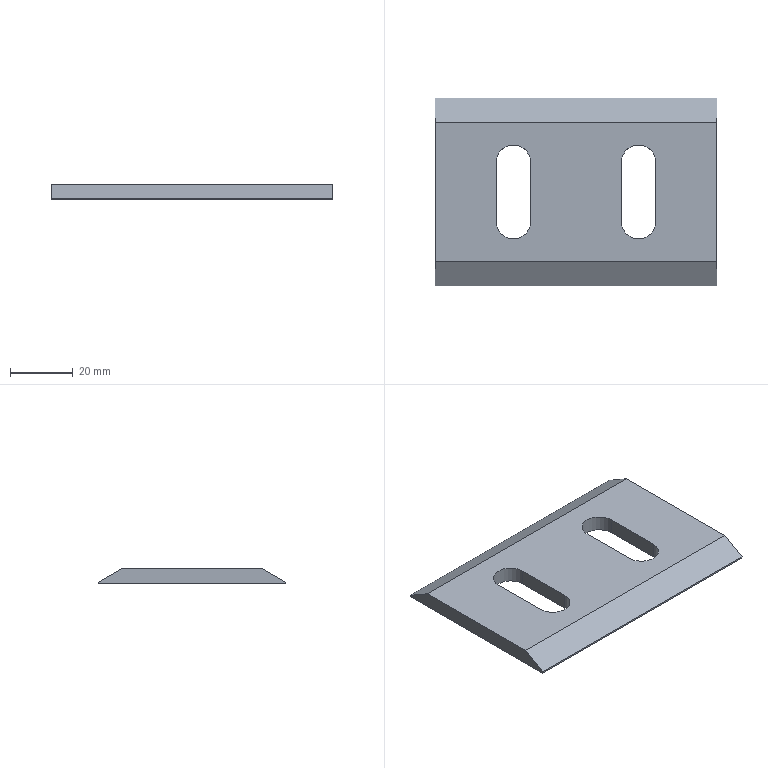Part | SolidWorks | features Chamfer 2, FlatPattern 1, SMBaseFlange 1, SheetMetal 1 | 1 solid | 16 faces | box 90 x 60 x 5 mm | volume 20803 mm3 | plane 12 | cylinder 4 | commonest cylinder face diameters 11 x4
STEP:
#1=CARTESIAN_POINT('',(0.,0.,-5.));
#2=VERTEX_POINT('',#1);
#3=CARTESIAN_POINT('',(0.,0.,-4.5));
#4=VERTEX_POINT('',#3);
#5=CARTESIAN_POINT('',(0.,0.,-5.));
#6=DIRECTION('',(0.,0.,1.));
#7=VECTOR('',#6,1000.);
#8=LINE('',#5,#7);
#9=EDGE_CURVE('',#2,#4,#8,.T.);
#10=ORIENTED_EDGE('',*,*,#9,.T.);
#11=CARTESIAN_POINT('',(0.,7.794,0.));
#12=VERTEX_POINT('',#11);
#13=CARTESIAN_POINT('',(0.,-0.2165,-4.625));
#14=DIRECTION('',(0.,0.866,0.5));
#15=VECTOR('',#14,1000.);
#16=LINE('',#13,#15);
#17=EDGE_CURVE('',#4,#12,#16,.T.);
#18=ORIENTED_EDGE('',*,*,#17,.T.);
#19=CARTESIAN_POINT('',(0.,52.206,0.));
#20=VERTEX_POINT('',#19);
#21=CARTESIAN_POINT('',(0.,0.,0.));
#22=DIRECTION('',(0.,-1.,0.));
#23=VECTOR('',#22,1000.);
#24=LINE('',#21,#23);
#25=EDGE_CURVE('',#20,#12,#24,.T.);
#26=ORIENTED_EDGE('',*,*,#25,.F.);
#27=CARTESIAN_POINT('',(0.,60.,-4.5));
#28=VERTEX_POINT('',#27);
#29=CARTESIAN_POINT('',(0.,15.217,21.356));
#30=DIRECTION('',(0.,0.866,-0.5));
#31=VECTOR('',#30,1000.);
#32=LINE('',#29,#31);
#33=EDGE_CURVE('',#20,#28,#32,.T.);
#34=ORIENTED_EDGE('',*,*,#33,.T.);
#35=CARTESIAN_POINT('',(0.,60.,-5.));
#36=VERTEX_POINT('',#35);
#37=CARTESIAN_POINT('',(0.,60.,-5.));
#38=DIRECTION('',(0.,0.,1.));
#39=VECTOR('',#38,1000.);
#40=LINE('',#37,#39);
#41=EDGE_CURVE('',#36,#28,#40,.T.);
#42=ORIENTED_EDGE('',*,*,#41,.F.);
#43=CARTESIAN_POINT('',(0.,0.,-5.));
#44=DIRECTION('',(0.,-1.,0.));
#45=VECTOR('',#44,1000.);
#46=LINE('',#43,#45);
#47=EDGE_CURVE('',#36,#2,#46,.T.);
#48=ORIENTED_EDGE('',*,*,#47,.T.);
#49=EDGE_LOOP('',(#10,#18,#26,#34,#42,#48));
#50=FACE_OUTER_BOUND('',#49,.T.);
#51=CARTESIAN_POINT('',(0.,0.,-5.));
#52=DIRECTION('',(-1.,0.,0.));
#53=DIRECTION('',(0.,0.,1.));
#54=AXIS2_PLACEMENT_3D('',#51,#52,#53);
#55=PLANE('',#54);
#56=ADVANCED_FACE('',(#50),#55,.T.);
#57=ORIENTED_EDGE('',*,*,#41,.T.);
#58=CARTESIAN_POINT('',(90.,60.,-4.5));
#59=VERTEX_POINT('',#58);
#60=CARTESIAN_POINT('',(90.,60.,-4.5));
#61=DIRECTION('',(1.,0.,0.));
#62=VECTOR('',#61,1000.);
#63=LINE('',#60,#62);
#64=EDGE_CURVE('',#28,#59,#63,.T.);
#65=ORIENTED_EDGE('',*,*,#64,.T.);
#66=CARTESIAN_POINT('',(90.,60.,-5.));
#67=VERTEX_POINT('',#66);
#68=CARTESIAN_POINT('',(90.,60.,-5.));
#69=DIRECTION('',(0.,0.,1.));
#70=VECTOR('',#69,1000.);
#71=LINE('',#68,#70);
#72=EDGE_CURVE('',#67,#59,#71,.T.);
#73=ORIENTED_EDGE('',*,*,#72,.F.);
#74=CARTESIAN_POINT('',(0.,60.,-5.));
#75=DIRECTION('',(-1.,0.,0.));
#76=VECTOR('',#75,1000.);
#77=LINE('',#74,#76);
#78=EDGE_CURVE('',#67,#36,#77,.T.);
#79=ORIENTED_EDGE('',*,*,#78,.T.);
#80=EDGE_LOOP('',(#57,#65,#73,#79));
#81=FACE_OUTER_BOUND('',#80,.T.);
#82=CARTESIAN_POINT('',(0.,60.,-5.));
#83=DIRECTION('',(0.,1.,0.));
#84=DIRECTION('',(0.,0.,1.));
#85=AXIS2_PLACEMENT_3D('',#82,#83,#84);
#86=PLANE('',#85);
#87=ADVANCED_FACE('',(#81),#86,.T.);
#88=CARTESIAN_POINT('',(90.,7.794,0.));
#89=VERTEX_POINT('',#88);
#90=CARTESIAN_POINT('',(90.,52.206,0.));
#91=VERTEX_POINT('',#90);
#92=CARTESIAN_POINT('',(90.,0.,0.));
#93=DIRECTION('',(0.,1.,0.));
#94=VECTOR('',#93,1000.);
#95=LINE('',#92,#94);
#96=EDGE_CURVE('',#89,#91,#95,.T.);
#97=ORIENTED_EDGE('',*,*,#96,.F.);
#98=CARTESIAN_POINT('',(90.,0.,-4.5));
#99=VERTEX_POINT('',#98);
#100=CARTESIAN_POINT('',(90.,-0.2165,-4.625));
#101=DIRECTION('',(0.,-0.866,-0.5));
#102=VECTOR('',#101,1000.);
#103=LINE('',#100,#102);
#104=EDGE_CURVE('',#89,#99,#103,.T.);
#105=ORIENTED_EDGE('',*,*,#104,.T.);
#106=CARTESIAN_POINT('',(90.,0.,-5.));
#107=VERTEX_POINT('',#106);
#108=CARTESIAN_POINT('',(90.,0.,-5.));
#109=DIRECTION('',(0.,0.,1.));
#110=VECTOR('',#109,1000.);
#111=LINE('',#108,#110);
#112=EDGE_CURVE('',#107,#99,#111,.T.);
#113=ORIENTED_EDGE('',*,*,#112,.F.);
#114=CARTESIAN_POINT('',(90.,0.,-5.));
#115=DIRECTION('',(0.,1.,0.));
#116=VECTOR('',#115,1000.);
#117=LINE('',#114,#116);
#118=EDGE_CURVE('',#107,#67,#117,.T.);
#119=ORIENTED_EDGE('',*,*,#118,.T.);
#120=ORIENTED_EDGE('',*,*,#72,.T.);
#121=CARTESIAN_POINT('',(90.,15.217,21.356));
#122=DIRECTION('',(0.,-0.866,0.5));
#123=VECTOR('',#122,1000.);
#124=LINE('',#121,#123);
#125=EDGE_CURVE('',#59,#91,#124,.T.);
#126=ORIENTED_EDGE('',*,*,#125,.T.);
#127=EDGE_LOOP('',(#97,#105,#113,#119,#120,#126));
#128=FACE_OUTER_BOUND('',#127,.T.);
#129=CARTESIAN_POINT('',(90.,0.,-5.));
#130=DIRECTION('',(1.,0.,0.));
#131=DIRECTION('',(0.,0.,-1.));
#132=AXIS2_PLACEMENT_3D('',#129,#130,#131);
#133=PLANE('',#132);
#134=ADVANCED_FACE('',(#128),#133,.T.);
#135=ORIENTED_EDGE('',*,*,#112,.T.);
#136=CARTESIAN_POINT('',(0.,0.,-4.5));
#137=DIRECTION('',(-1.,0.,0.));
#138=VECTOR('',#137,1000.);
#139=LINE('',#136,#138);
#140=EDGE_CURVE('',#99,#4,#139,.T.);
#141=ORIENTED_EDGE('',*,*,#140,.T.);
#142=ORIENTED_EDGE('',*,*,#9,.F.);
#143=CARTESIAN_POINT('',(0.,0.,-5.));
#144=DIRECTION('',(1.,0.,0.));
#145=VECTOR('',#144,1000.);
#146=LINE('',#143,#145);
#147=EDGE_CURVE('',#2,#107,#146,.T.);
#148=ORIENTED_EDGE('',*,*,#147,.T.);
#149=EDGE_LOOP('',(#135,#141,#142,#148));
#150=FACE_OUTER_BOUND('',#149,.T.);
#151=CARTESIAN_POINT('',(0.,0.,-5.));
#152=DIRECTION('',(0.,-1.,0.));
#153=DIRECTION('',(0.,0.,-1.));
#154=AXIS2_PLACEMENT_3D('',#151,#152,#153);
#155=PLANE('',#154);
#156=ADVANCED_FACE('',(#150),#155,.T.);
#157=CARTESIAN_POINT('',(70.5,39.5,-5.));
#158=VERTEX_POINT('',#157);
#159=CARTESIAN_POINT('',(59.5,39.5,-5.));
#160=VERTEX_POINT('',#159);
#161=CARTESIAN_POINT('',(65.,39.5,-5.));
#162=DIRECTION('',(0.,0.,1.));
#163=DIRECTION('',(1.,0.,0.));
#164=AXIS2_PLACEMENT_3D('',#161,#162,#163);
#165=CIRCLE('',#164,5.5);
#166=EDGE_CURVE('',#158,#160,#165,.T.);
#167=ORIENTED_EDGE('',*,*,#166,.T.);
#168=CARTESIAN_POINT('',(59.5,20.5,-5.));
#169=VERTEX_POINT('',#168);
#170=CARTESIAN_POINT('',(59.5,39.5,-5.));
#171=DIRECTION('',(0.,-1.,0.));
#172=VECTOR('',#171,1000.);
#173=LINE('',#170,#172);
#174=EDGE_CURVE('',#160,#169,#173,.T.);
#175=ORIENTED_EDGE('',*,*,#174,.T.);
#176=CARTESIAN_POINT('',(70.5,20.5,-5.));
#177=VERTEX_POINT('',#176);
#178=CARTESIAN_POINT('',(65.,20.5,-5.));
#179=DIRECTION('',(0.,0.,1.));
#180=DIRECTION('',(1.,0.,0.));
#181=AXIS2_PLACEMENT_3D('',#178,#179,#180);
#182=CIRCLE('',#181,5.5);
#183=EDGE_CURVE('',#169,#177,#182,.T.);
#184=ORIENTED_EDGE('',*,*,#183,.T.);
#185=CARTESIAN_POINT('',(70.5,39.5,-5.));
#186=DIRECTION('',(0.,1.,0.));
#187=VECTOR('',#186,1000.);
#188=LINE('',#185,#187);
#189=EDGE_CURVE('',#177,#158,#188,.T.);
#190=ORIENTED_EDGE('',*,*,#189,.T.);
#191=EDGE_LOOP('',(#167,#175,#184,#190));
#192=FACE_BOUND('',#191,.T.);
#193=CARTESIAN_POINT('',(30.5,39.5,-5.));
#194=VERTEX_POINT('',#193);
#195=CARTESIAN_POINT('',(19.5,39.5,-5.));
#196=VERTEX_POINT('',#195);
#197=CARTESIAN_POINT('',(25.,39.5,-5.));
#198=DIRECTION('',(0.,0.,1.));
#199=DIRECTION('',(1.,0.,0.));
#200=AXIS2_PLACEMENT_3D('',#197,#198,#199);
#201=CIRCLE('',#200,5.5);
#202=EDGE_CURVE('',#194,#196,#201,.T.);
#203=ORIENTED_EDGE('',*,*,#202,.T.);
#204=CARTESIAN_POINT('',(19.5,20.5,-5.));
#205=VERTEX_POINT('',#204);
#206=CARTESIAN_POINT('',(19.5,39.5,-5.));
#207=DIRECTION('',(0.,-1.,0.));
#208=VECTOR('',#207,1000.);
#209=LINE('',#206,#208);
#210=EDGE_CURVE('',#196,#205,#209,.T.);
#211=ORIENTED_EDGE('',*,*,#210,.T.);
#212=CARTESIAN_POINT('',(30.5,20.5,-5.));
#213=VERTEX_POINT('',#212);
#214=CARTESIAN_POINT('',(25.,20.5,-5.));
#215=DIRECTION('',(0.,0.,1.));
#216=DIRECTION('',(1.,0.,0.));
#217=AXIS2_PLACEMENT_3D('',#214,#215,#216);
#218=CIRCLE('',#217,5.5);
#219=EDGE_CURVE('',#205,#213,#218,.T.);
#220=ORIENTED_EDGE('',*,*,#219,.T.);
#221=CARTESIAN_POINT('',(30.5,39.5,-5.));
#222=DIRECTION('',(0.,1.,0.));
#223=VECTOR('',#222,1000.);
#224=LINE('',#221,#223);
#225=EDGE_CURVE('',#213,#194,#224,.T.);
#226=ORIENTED_EDGE('',*,*,#225,.T.);
#227=EDGE_LOOP('',(#203,#211,#220,#226));
#228=FACE_BOUND('',#227,.T.);
#229=ORIENTED_EDGE('',*,*,#47,.F.);
#230=ORIENTED_EDGE('',*,*,#78,.F.);
#231=ORIENTED_EDGE('',*,*,#118,.F.);
#232=ORIENTED_EDGE('',*,*,#147,.F.);
#233=EDGE_LOOP('',(#229,#230,#231,#232));
#234=FACE_OUTER_BOUND('',#233,.T.);
#235=CARTESIAN_POINT('',(0.,0.,-5.));
#236=DIRECTION('',(0.,0.,-1.));
#237=DIRECTION('',(-1.,0.,0.));
#238=AXIS2_PLACEMENT_3D('',#235,#236,#237);
#239=PLANE('',#238);
#240=ADVANCED_FACE('',(#192,#228,#234),#239,.T.);
#241=CARTESIAN_POINT('',(59.5,39.5,0.));
#242=VERTEX_POINT('',#241);
#243=CARTESIAN_POINT('',(59.5,20.5,0.));
#244=VERTEX_POINT('',#243);
#245=CARTESIAN_POINT('',(59.5,39.5,0.));
#246=DIRECTION('',(0.,-1.,0.));
#247=VECTOR('',#246,1000.);
#248=LINE('',#245,#247);
#249=EDGE_CURVE('',#242,#244,#248,.T.);
#250=ORIENTED_EDGE('',*,*,#249,.F.);
#251=CARTESIAN_POINT('',(70.5,39.5,0.));
#252=VERTEX_POINT('',#251);
#253=CARTESIAN_POINT('',(65.,39.5,0.));
#254=DIRECTION('',(0.,0.,1.));
#255=DIRECTION('',(1.,0.,0.));
#256=AXIS2_PLACEMENT_3D('',#253,#254,#255);
#257=CIRCLE('',#256,5.5);
#258=EDGE_CURVE('',#252,#242,#257,.T.);
#259=ORIENTED_EDGE('',*,*,#258,.F.);
#260=CARTESIAN_POINT('',(70.5,20.5,0.));
#261=VERTEX_POINT('',#260);
#262=CARTESIAN_POINT('',(70.5,39.5,0.));
#263=DIRECTION('',(0.,1.,0.));
#264=VECTOR('',#263,1000.);
#265=LINE('',#262,#264);
#266=EDGE_CURVE('',#261,#252,#265,.T.);
#267=ORIENTED_EDGE('',*,*,#266,.F.);
#268=CARTESIAN_POINT('',(65.,20.5,0.));
#269=DIRECTION('',(0.,0.,1.));
#270=DIRECTION('',(1.,0.,0.));
#271=AXIS2_PLACEMENT_3D('',#268,#269,#270);
#272=CIRCLE('',#271,5.5);
#273=EDGE_CURVE('',#244,#261,#272,.T.);
#274=ORIENTED_EDGE('',*,*,#273,.F.);
#275=EDGE_LOOP('',(#250,#259,#267,#274));
#276=FACE_BOUND('',#275,.T.);
#277=CARTESIAN_POINT('',(19.5,39.5,0.));
#278=VERTEX_POINT('',#277);
#279=CARTESIAN_POINT('',(19.5,20.5,0.));
#280=VERTEX_POINT('',#279);
#281=CARTESIAN_POINT('',(19.5,39.5,0.));
#282=DIRECTION('',(0.,-1.,0.));
#283=VECTOR('',#282,1000.);
#284=LINE('',#281,#283);
#285=EDGE_CURVE('',#278,#280,#284,.T.);
#286=ORIENTED_EDGE('',*,*,#285,.F.);
#287=CARTESIAN_POINT('',(30.5,39.5,0.));
#288=VERTEX_POINT('',#287);
#289=CARTESIAN_POINT('',(25.,39.5,0.));
#290=DIRECTION('',(0.,0.,1.));
#291=DIRECTION('',(1.,0.,0.));
#292=AXIS2_PLACEMENT_3D('',#289,#290,#291);
#293=CIRCLE('',#292,5.5);
#294=EDGE_CURVE('',#288,#278,#293,.T.);
#295=ORIENTED_EDGE('',*,*,#294,.F.);
#296=CARTESIAN_POINT('',(30.5,20.5,0.));
#297=VERTEX_POINT('',#296);
#298=CARTESIAN_POINT('',(30.5,39.5,0.));
#299=DIRECTION('',(0.,1.,0.));
#300=VECTOR('',#299,1000.);
#301=LINE('',#298,#300);
#302=EDGE_CURVE('',#297,#288,#301,.T.);
#303=ORIENTED_EDGE('',*,*,#302,.F.);
#304=CARTESIAN_POINT('',(25.,20.5,0.));
#305=DIRECTION('',(0.,0.,1.));
#306=DIRECTION('',(1.,0.,0.));
#307=AXIS2_PLACEMENT_3D('',#304,#305,#306);
#308=CIRCLE('',#307,5.5);
#309=EDGE_CURVE('',#280,#297,#308,.T.);
#310=ORIENTED_EDGE('',*,*,#309,.F.);
#311=EDGE_LOOP('',(#286,#295,#303,#310));
#312=FACE_BOUND('',#311,.T.);
#313=ORIENTED_EDGE('',*,*,#25,.T.);
#314=CARTESIAN_POINT('',(90.,7.794,0.));
#315=DIRECTION('',(1.,0.,0.));
#316=VECTOR('',#315,1000.);
#317=LINE('',#314,#316);
#318=EDGE_CURVE('',#12,#89,#317,.T.);
#319=ORIENTED_EDGE('',*,*,#318,.T.);
#320=ORIENTED_EDGE('',*,*,#96,.T.);
#321=CARTESIAN_POINT('',(0.,52.206,0.));
#322=DIRECTION('',(-1.,0.,0.));
#323=VECTOR('',#322,1000.);
#324=LINE('',#321,#323);
#325=EDGE_CURVE('',#91,#20,#324,.T.);
#326=ORIENTED_EDGE('',*,*,#325,.T.);
#327=EDGE_LOOP('',(#313,#319,#320,#326));
#328=FACE_OUTER_BOUND('',#327,.T.);
#329=CARTESIAN_POINT('',(0.,0.,0.));
#330=DIRECTION('',(0.,0.,-1.));
#331=DIRECTION('',(-1.,0.,0.));
#332=AXIS2_PLACEMENT_3D('',#329,#330,#331);
#333=PLANE('',#332);
#334=ADVANCED_FACE('',(#276,#312,#328),#333,.F.);
#335=ORIENTED_EDGE('',*,*,#294,.T.);
#336=CARTESIAN_POINT('',(19.5,39.5,-5.));
#337=DIRECTION('',(0.,0.,1.));
#338=VECTOR('',#337,1000.);
#339=LINE('',#336,#338);
#340=EDGE_CURVE('',#196,#278,#339,.T.);
#341=ORIENTED_EDGE('',*,*,#340,.F.);
#342=ORIENTED_EDGE('',*,*,#202,.F.);
#343=CARTESIAN_POINT('',(30.5,39.5,-5.));
#344=DIRECTION('',(0.,0.,1.));
#345=VECTOR('',#344,1000.);
#346=LINE('',#343,#345);
#347=EDGE_CURVE('',#194,#288,#346,.T.);
#348=ORIENTED_EDGE('',*,*,#347,.T.);
#349=EDGE_LOOP('',(#335,#341,#342,#348));
#350=FACE_OUTER_BOUND('',#349,.T.);
#351=CARTESIAN_POINT('',(25.,39.5,-5.));
#352=DIRECTION('',(0.,0.,1.));
#353=DIRECTION('',(1.,0.,0.));
#354=AXIS2_PLACEMENT_3D('',#351,#352,#353);
#355=CYLINDRICAL_SURFACE('',#354,5.5);
#356=ADVANCED_FACE('',(#350),#355,.F.);
#357=ORIENTED_EDGE('',*,*,#302,.T.);
#358=ORIENTED_EDGE('',*,*,#347,.F.);
#359=ORIENTED_EDGE('',*,*,#225,.F.);
#360=CARTESIAN_POINT('',(30.5,20.5,-5.));
#361=DIRECTION('',(0.,0.,1.));
#362=VECTOR('',#361,1000.);
#363=LINE('',#360,#362);
#364=EDGE_CURVE('',#213,#297,#363,.T.);
#365=ORIENTED_EDGE('',*,*,#364,.T.);
#366=EDGE_LOOP('',(#357,#358,#359,#365));
#367=FACE_OUTER_BOUND('',#366,.T.);
#368=CARTESIAN_POINT('',(30.5,39.5,-5.));
#369=DIRECTION('',(1.,0.,0.));
#370=DIRECTION('',(0.,0.,-1.));
#371=AXIS2_PLACEMENT_3D('',#368,#369,#370);
#372=PLANE('',#371);
#373=ADVANCED_FACE('',(#367),#372,.F.);
#374=ORIENTED_EDGE('',*,*,#309,.T.);
#375=ORIENTED_EDGE('',*,*,#364,.F.);
#376=ORIENTED_EDGE('',*,*,#219,.F.);
#377=CARTESIAN_POINT('',(19.5,20.5,-5.));
#378=DIRECTION('',(0.,0.,1.));
#379=VECTOR('',#378,1000.);
#380=LINE('',#377,#379);
#381=EDGE_CURVE('',#205,#280,#380,.T.);
#382=ORIENTED_EDGE('',*,*,#381,.T.);
#383=EDGE_LOOP('',(#374,#375,#376,#382));
#384=FACE_OUTER_BOUND('',#383,.T.);
#385=CARTESIAN_POINT('',(25.,20.5,-5.));
#386=DIRECTION('',(0.,0.,1.));
#387=DIRECTION('',(1.,0.,0.));
#388=AXIS2_PLACEMENT_3D('',#385,#386,#387);
#389=CYLINDRICAL_SURFACE('',#388,5.5);
#390=ADVANCED_FACE('',(#384),#389,.F.);
#391=ORIENTED_EDGE('',*,*,#285,.T.);
#392=ORIENTED_EDGE('',*,*,#381,.F.);
#393=ORIENTED_EDGE('',*,*,#210,.F.);
#394=ORIENTED_EDGE('',*,*,#340,.T.);
#395=EDGE_LOOP('',(#391,#392,#393,#394));
#396=FACE_OUTER_BOUND('',#395,.T.);
#397=CARTESIAN_POINT('',(19.5,39.5,-5.));
#398=DIRECTION('',(-1.,0.,0.));
#399=DIRECTION('',(0.,0.,1.));
#400=AXIS2_PLACEMENT_3D('',#397,#398,#399);
#401=PLANE('',#400);
#402=ADVANCED_FACE('',(#396),#401,.F.);
#403=ORIENTED_EDGE('',*,*,#258,.T.);
#404=CARTESIAN_POINT('',(59.5,39.5,-5.));
#405=DIRECTION('',(0.,0.,1.));
#406=VECTOR('',#405,1000.);
#407=LINE('',#404,#406);
#408=EDGE_CURVE('',#160,#242,#407,.T.);
#409=ORIENTED_EDGE('',*,*,#408,.F.);
#410=ORIENTED_EDGE('',*,*,#166,.F.);
#411=CARTESIAN_POINT('',(70.5,39.5,-5.));
#412=DIRECTION('',(0.,0.,1.));
#413=VECTOR('',#412,1000.);
#414=LINE('',#411,#413);
#415=EDGE_CURVE('',#158,#252,#414,.T.);
#416=ORIENTED_EDGE('',*,*,#415,.T.);
#417=EDGE_LOOP('',(#403,#409,#410,#416));
#418=FACE_OUTER_BOUND('',#417,.T.);
#419=CARTESIAN_POINT('',(65.,39.5,-5.));
#420=DIRECTION('',(0.,0.,1.));
#421=DIRECTION('',(1.,0.,0.));
#422=AXIS2_PLACEMENT_3D('',#419,#420,#421);
#423=CYLINDRICAL_SURFACE('',#422,5.5);
#424=ADVANCED_FACE('',(#418),#423,.F.);
#425=ORIENTED_EDGE('',*,*,#266,.T.);
#426=ORIENTED_EDGE('',*,*,#415,.F.);
#427=ORIENTED_EDGE('',*,*,#189,.F.);
#428=CARTESIAN_POINT('',(70.5,20.5,-5.));
#429=DIRECTION('',(0.,0.,1.));
#430=VECTOR('',#429,1000.);
#431=LINE('',#428,#430);
#432=EDGE_CURVE('',#177,#261,#431,.T.);
#433=ORIENTED_EDGE('',*,*,#432,.T.);
#434=EDGE_LOOP('',(#425,#426,#427,#433));
#435=FACE_OUTER_BOUND('',#434,.T.);
#436=CARTESIAN_POINT('',(70.5,39.5,-5.));
#437=DIRECTION('',(1.,0.,0.));
#438=DIRECTION('',(0.,0.,-1.));
#439=AXIS2_PLACEMENT_3D('',#436,#437,#438);
#440=PLANE('',#439);
#441=ADVANCED_FACE('',(#435),#440,.F.);
#442=ORIENTED_EDGE('',*,*,#273,.T.);
#443=ORIENTED_EDGE('',*,*,#432,.F.);
#444=ORIENTED_EDGE('',*,*,#183,.F.);
#445=CARTESIAN_POINT('',(59.5,20.5,-5.));
#446=DIRECTION('',(0.,0.,1.));
#447=VECTOR('',#446,1000.);
#448=LINE('',#445,#447);
#449=EDGE_CURVE('',#169,#244,#448,.T.);
#450=ORIENTED_EDGE('',*,*,#449,.T.);
#451=EDGE_LOOP('',(#442,#443,#444,#450));
#452=FACE_OUTER_BOUND('',#451,.T.);
#453=CARTESIAN_POINT('',(65.,20.5,-5.));
#454=DIRECTION('',(0.,0.,1.));
#455=DIRECTION('',(1.,0.,0.));
#456=AXIS2_PLACEMENT_3D('',#453,#454,#455);
#457=CYLINDRICAL_SURFACE('',#456,5.5);
#458=ADVANCED_FACE('',(#452),#457,.F.);
#459=ORIENTED_EDGE('',*,*,#249,.T.);
#460=ORIENTED_EDGE('',*,*,#449,.F.);
#461=ORIENTED_EDGE('',*,*,#174,.F.);
#462=ORIENTED_EDGE('',*,*,#408,.T.);
#463=EDGE_LOOP('',(#459,#460,#461,#462));
#464=FACE_OUTER_BOUND('',#463,.T.);
#465=CARTESIAN_POINT('',(59.5,39.5,-5.));
#466=DIRECTION('',(-1.,0.,0.));
#467=DIRECTION('',(0.,-1.,0.));
#468=AXIS2_PLACEMENT_3D('',#465,#466,#467);
#469=PLANE('',#468);
#470=ADVANCED_FACE('',(#464),#469,.F.);
#471=ORIENTED_EDGE('',*,*,#125,.F.);
#472=ORIENTED_EDGE('',*,*,#64,.F.);
#473=ORIENTED_EDGE('',*,*,#33,.F.);
#474=ORIENTED_EDGE('',*,*,#325,.F.);
#475=EDGE_LOOP('',(#471,#472,#473,#474));
#476=FACE_OUTER_BOUND('',#475,.T.);
#477=CARTESIAN_POINT('',(0.,52.206,0.));
#478=DIRECTION('',(0.,0.5,0.866));
#479=DIRECTION('',(1.,0.,0.));
#480=AXIS2_PLACEMENT_3D('',#477,#478,#479);
#481=PLANE('',#480);
#482=ADVANCED_FACE('',(#476),#481,.T.);
#483=ORIENTED_EDGE('',*,*,#17,.F.);
#484=ORIENTED_EDGE('',*,*,#140,.F.);
#485=ORIENTED_EDGE('',*,*,#104,.F.);
#486=ORIENTED_EDGE('',*,*,#318,.F.);
#487=EDGE_LOOP('',(#483,#484,#485,#486));
#488=FACE_OUTER_BOUND('',#487,.T.);
#489=CARTESIAN_POINT('',(0.,7.794,0.));
#490=DIRECTION('',(0.,-0.5,0.866));
#491=DIRECTION('',(-1.,0.,0.));
#492=AXIS2_PLACEMENT_3D('',#489,#490,#491);
#493=PLANE('',#492);
#494=ADVANCED_FACE('',(#488),#493,.T.);
#495=CLOSED_SHELL('',(#56,#87,#134,#156,#240,#334,#356,#373,#390,#402,#424,#441,#458,#470,#482,#494));
#496=MANIFOLD_SOLID_BREP('',#495);
#497=CARTESIAN_POINT('',(0.,0.,0.));
#498=DIRECTION('',(0.,0.,1.));
#499=DIRECTION('',(1.,0.,0.));
#500=AXIS2_PLACEMENT_3D('',#497,#498,#499);
#501=(LENGTH_UNIT()NAMED_UNIT(*)SI_UNIT(.MILLI.,.METRE.));
#502=UNCERTAINTY_MEASURE_WITH_UNIT(LENGTH_MEASURE(0.00001),#501,'','');
#503=(NAMED_UNIT(*)PLANE_ANGLE_UNIT()SI_UNIT($,.RADIAN.));
#504=(NAMED_UNIT(*)SI_UNIT($,.STERADIAN.)SOLID_ANGLE_UNIT());
#505=(GEOMETRIC_REPRESENTATION_CONTEXT(3)GLOBAL_UNCERTAINTY_ASSIGNED_CONTEXT((#502))GLOBAL_UNIT_ASSIGNED_CONTEXT((#501,#503,#504))REPRESENTATION_CONTEXT('',''));
#506=ADVANCED_BREP_SHAPE_REPRESENTATION('',(#496,#500),#505);